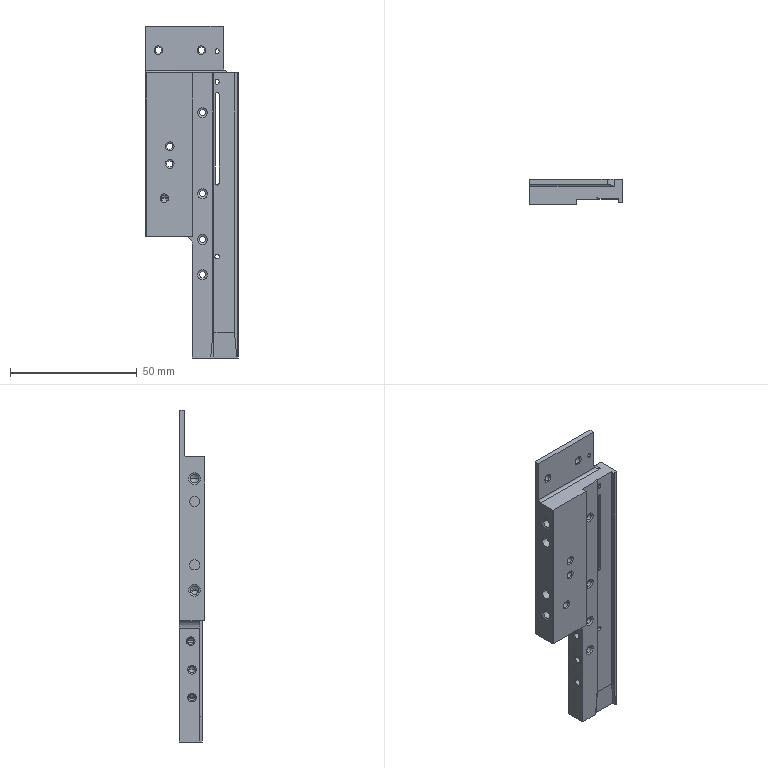Part | NX | 1 solid | 120 faces | box 36.55 x 10 x 131 mm | volume 27718 mm3 | cylinder 46 | cone 40 | plane 34 | commonest cylinder face diameters 2.5 x24 1.5 x9 3.3 x4 4 x4 1.8 x2 6 x2